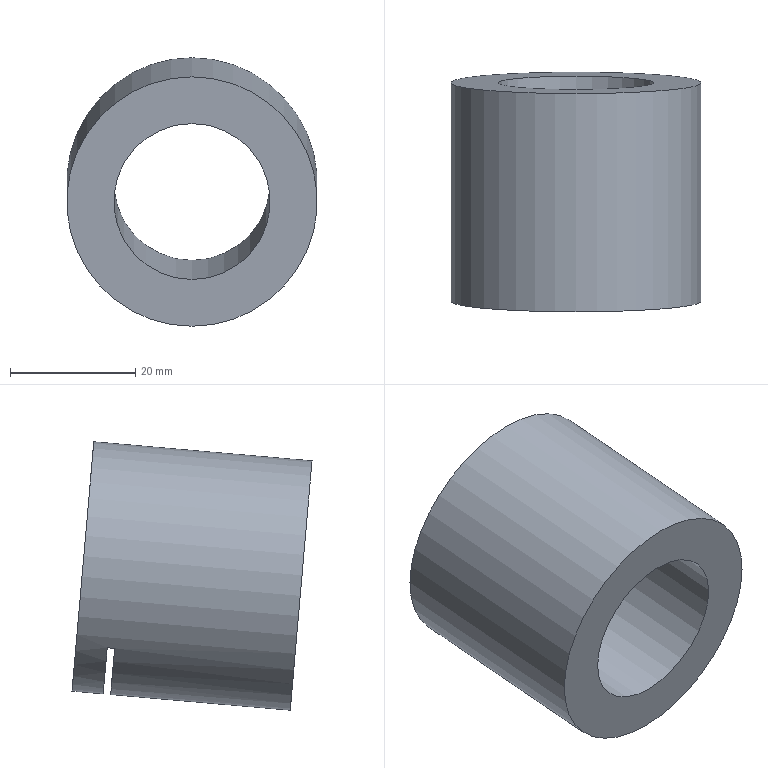Part | NX | features solid 2 | 1 solid | 7 faces | box 40 x 38.353 x 42.898 mm | volume 26610 mm3 | plane 5 | cylinder 2 | commonest cylinder face diameters 25 x1 40 x1
STEP:
#1=CARTESIAN_POINT('',(-150.187,110.375,-13.16));
#2=VERTEX_POINT('',#1);
#3=CARTESIAN_POINT('',(-150.187,112.118,-33.084));
#4=DIRECTION('',(0.,0.9962,0.08716));
#5=DIRECTION('',(0.,-0.08716,0.9962));
#6=AXIS2_PLACEMENT_3D('',#3,#4,#5);
#7=CIRCLE('',#6,20.);
#8=EDGE_CURVE('',#2,#2,#7,.T.);
#9=ORIENTED_EDGE('',*,*,#8,.F.);
#10=EDGE_LOOP('',(#9));
#11=FACE_BOUND('',#10,.T.);
#12=CARTESIAN_POINT('',(-150.187,78.994,-56.059));
#13=VERTEX_POINT('',#12);
#14=CARTESIAN_POINT('',(-150.187,77.251,-36.135));
#15=DIRECTION('',(0.,-0.9962,-0.08716));
#16=DIRECTION('',(0.,0.08716,-0.9962));
#17=AXIS2_PLACEMENT_3D('',#14,#15,#16);
#18=CIRCLE('',#17,20.);
#19=EDGE_CURVE('',#13,#13,#18,.F.);
#20=ORIENTED_EDGE('',*,*,#19,.T.);
#21=EDGE_LOOP('',(#20));
#22=FACE_BOUND('',#21,.T.);
#23=CARTESIAN_POINT('',(-165.719,108.235,-46.072));
#24=VERTEX_POINT('',#23);
#25=CARTESIAN_POINT('',(-165.719,107.04,-46.177));
#26=VERTEX_POINT('',#25);
#27=CARTESIAN_POINT('',(-165.719,71.376,-49.297));
#28=DIRECTION('',(0.,0.9962,0.08716));
#29=VECTOR('',#28,1000.);
#30=LINE('',#27,#29);
#31=EDGE_CURVE('',#24,#26,#30,.F.);
#32=ORIENTED_EDGE('',*,*,#31,.T.);
#33=CARTESIAN_POINT('',(-134.656,107.04,-46.177));
#34=VERTEX_POINT('',#33);
#35=CARTESIAN_POINT('',(-150.187,105.942,-33.625));
#36=DIRECTION('',(0.,0.9962,0.08716));
#37=DIRECTION('',(0.,-0.08716,0.9962));
#38=AXIS2_PLACEMENT_3D('',#35,#36,#37);
#39=CIRCLE('',#38,20.);
#40=EDGE_CURVE('',#26,#34,#39,.F.);
#41=ORIENTED_EDGE('',*,*,#40,.T.);
#42=CARTESIAN_POINT('',(-134.656,108.235,-46.072));
#43=VERTEX_POINT('',#42);
#44=CARTESIAN_POINT('',(-134.656,71.376,-49.297));
#45=DIRECTION('',(0.,0.9962,0.08716));
#46=VECTOR('',#45,1000.);
#47=LINE('',#44,#46);
#48=EDGE_CURVE('',#34,#43,#47,.T.);
#49=ORIENTED_EDGE('',*,*,#48,.T.);
#50=CARTESIAN_POINT('',(-150.187,107.137,-33.52));
#51=DIRECTION('',(0.,0.9962,0.08716));
#52=DIRECTION('',(0.,-0.08716,0.9962));
#53=AXIS2_PLACEMENT_3D('',#50,#51,#52);
#54=CIRCLE('',#53,20.);
#55=EDGE_CURVE('',#24,#43,#54,.F.);
#56=ORIENTED_EDGE('',*,*,#55,.F.);
#57=EDGE_LOOP('',(#32,#41,#49,#56));
#58=FACE_BOUND('',#57,.T.);
#59=CARTESIAN_POINT('',(-150.187,112.118,-33.084));
#60=DIRECTION('',(0.,-0.9962,-0.08716));
#61=DIRECTION('',(0.,0.08716,-0.9962));
#62=AXIS2_PLACEMENT_3D('',#59,#60,#61);
#63=CYLINDRICAL_SURFACE('',#62,20.);
#64=ADVANCED_FACE('',(#11,#22,#58),#63,.T.);
#65=CARTESIAN_POINT('',(-150.187,111.028,-20.632));
#66=VERTEX_POINT('',#65);
#67=CARTESIAN_POINT('',(-150.187,112.118,-33.084));
#68=DIRECTION('',(0.,0.9962,0.08716));
#69=DIRECTION('',(0.,-0.08716,0.9962));
#70=AXIS2_PLACEMENT_3D('',#67,#68,#69);
#71=CIRCLE('',#70,12.5);
#72=EDGE_CURVE('',#66,#66,#71,.T.);
#73=ORIENTED_EDGE('',*,*,#72,.F.);
#74=EDGE_LOOP('',(#73));
#75=FACE_BOUND('',#74,.T.);
#76=ORIENTED_EDGE('',*,*,#8,.T.);
#77=EDGE_LOOP('',(#76));
#78=FACE_BOUND('',#77,.T.);
#79=CARTESIAN_POINT('',(-150.187,112.118,-33.084));
#80=DIRECTION('',(0.,0.9962,0.08716));
#81=DIRECTION('',(1.,0.,0.));
#82=AXIS2_PLACEMENT_3D('',#79,#80,#81);
#83=PLANE('',#82);
#84=ADVANCED_FACE('',(#75,#78),#83,.T.);
#85=CARTESIAN_POINT('',(-150.187,78.341,-48.587));
#86=VERTEX_POINT('',#85);
#87=CARTESIAN_POINT('',(-150.187,77.251,-36.135));
#88=DIRECTION('',(0.,-0.9962,-0.08716));
#89=DIRECTION('',(0.,0.08716,-0.9962));
#90=AXIS2_PLACEMENT_3D('',#87,#88,#89);
#91=CIRCLE('',#90,12.5);
#92=EDGE_CURVE('',#86,#86,#91,.F.);
#93=ORIENTED_EDGE('',*,*,#92,.T.);
#94=EDGE_LOOP('',(#93));
#95=FACE_BOUND('',#94,.T.);
#96=ORIENTED_EDGE('',*,*,#19,.F.);
#97=EDGE_LOOP('',(#96));
#98=FACE_BOUND('',#97,.T.);
#99=CARTESIAN_POINT('',(-150.187,77.251,-36.135));
#100=DIRECTION('',(0.,-0.9962,-0.08716));
#101=DIRECTION('',(0.,0.08716,-0.9962));
#102=AXIS2_PLACEMENT_3D('',#99,#100,#101);
#103=PLANE('',#102);
#104=ADVANCED_FACE('',(#95,#98),#103,.T.);
#105=ORIENTED_EDGE('',*,*,#72,.T.);
#106=EDGE_LOOP('',(#105));
#107=FACE_BOUND('',#106,.T.);
#108=ORIENTED_EDGE('',*,*,#92,.F.);
#109=EDGE_LOOP('',(#108));
#110=FACE_BOUND('',#109,.T.);
#111=CARTESIAN_POINT('',(-150.187,77.45,-36.117));
#112=DIRECTION('',(0.,0.9962,0.08716));
#113=DIRECTION('',(0.,-0.08716,0.9962));
#114=AXIS2_PLACEMENT_3D('',#111,#112,#113);
#115=CYLINDRICAL_SURFACE('',#114,12.5);
#116=ADVANCED_FACE('',(#107,#110),#115,.F.);
#117=CARTESIAN_POINT('',(-134.575,107.04,-46.177));
#118=DIRECTION('',(1.,0.,0.));
#119=VECTOR('',#118,1000.);
#120=LINE('',#117,#119);
#121=EDGE_CURVE('',#34,#26,#120,.F.);
#122=ORIENTED_EDGE('',*,*,#121,.F.);
#123=ORIENTED_EDGE('',*,*,#40,.F.);
#124=EDGE_LOOP('',(#122,#123));
#125=FACE_BOUND('',#124,.T.);
#126=CARTESIAN_POINT('',(-134.575,111.397,-95.986));
#127=DIRECTION('',(0.,0.9962,0.08716));
#128=DIRECTION('',(0.,-0.08716,0.9962));
#129=AXIS2_PLACEMENT_3D('',#126,#127,#128);
#130=PLANE('',#129);
#131=ADVANCED_FACE('',(#125),#130,.T.);
#132=ORIENTED_EDGE('',*,*,#55,.T.);
#133=CARTESIAN_POINT('',(-134.575,108.235,-46.072));
#134=DIRECTION('',(1.,0.,0.));
#135=VECTOR('',#134,1000.);
#136=LINE('',#133,#135);
#137=EDGE_CURVE('',#43,#24,#136,.F.);
#138=ORIENTED_EDGE('',*,*,#137,.T.);
#139=EDGE_LOOP('',(#132,#138));
#140=FACE_BOUND('',#139,.T.);
#141=CARTESIAN_POINT('',(-134.575,112.593,-95.882));
#142=DIRECTION('',(0.,0.9962,0.08716));
#143=DIRECTION('',(0.,-0.08716,0.9962));
#144=AXIS2_PLACEMENT_3D('',#141,#142,#143);
#145=PLANE('',#144);
#146=ADVANCED_FACE('',(#140),#145,.F.);
#147=ORIENTED_EDGE('',*,*,#121,.T.);
#148=ORIENTED_EDGE('',*,*,#31,.F.);
#149=ORIENTED_EDGE('',*,*,#137,.F.);
#150=ORIENTED_EDGE('',*,*,#48,.F.);
#151=EDGE_LOOP('',(#147,#148,#149,#150));
#152=FACE_BOUND('',#151,.T.);
#153=CARTESIAN_POINT('',(-134.575,108.235,-46.072));
#154=DIRECTION('',(0.,-0.08716,0.9962));
#155=DIRECTION('',(0.,-0.9962,-0.08716));
#156=AXIS2_PLACEMENT_3D('',#153,#154,#155);
#157=PLANE('',#156);
#158=ADVANCED_FACE('',(#152),#157,.F.);
#159=CLOSED_SHELL('',(#64,#84,#104,#116,#131,#146,#158));
#160=MANIFOLD_SOLID_BREP('',#159);
#161=(LENGTH_UNIT()NAMED_UNIT(*)SI_UNIT(.MILLI.,.METRE.));
#162=UNCERTAINTY_MEASURE_WITH_UNIT(LENGTH_MEASURE(0.00001),#161,'','');
#163=(NAMED_UNIT(*)PLANE_ANGLE_UNIT()SI_UNIT($,.RADIAN.));
#164=(NAMED_UNIT(*)SI_UNIT($,.STERADIAN.)SOLID_ANGLE_UNIT());
#165=(GEOMETRIC_REPRESENTATION_CONTEXT(3)GLOBAL_UNCERTAINTY_ASSIGNED_CONTEXT((#162))GLOBAL_UNIT_ASSIGNED_CONTEXT((#161,#163,#164))REPRESENTATION_CONTEXT('',''));
#166=ADVANCED_BREP_SHAPE_REPRESENTATION('',(#160),#165);